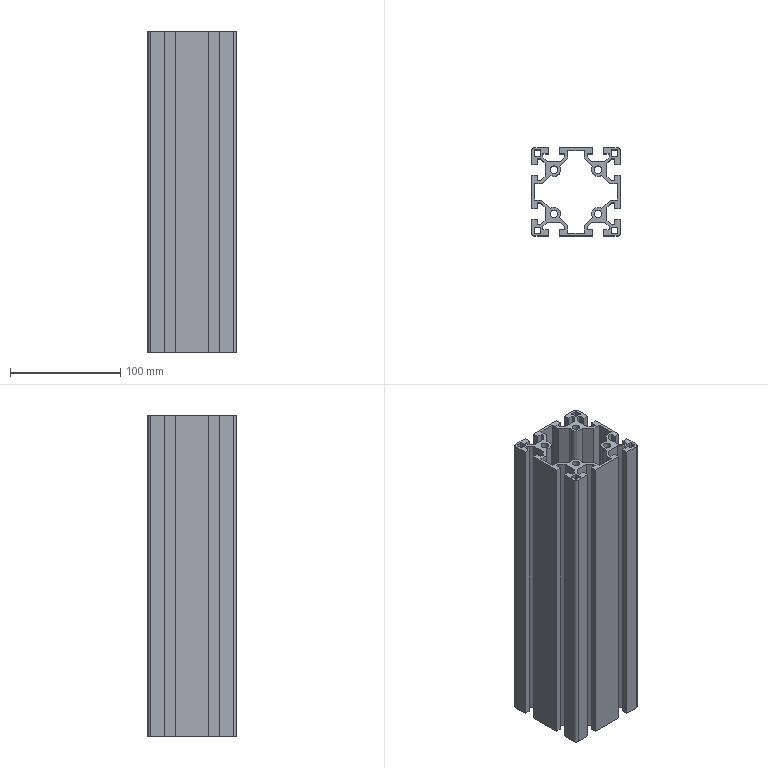Part | NX | 1 solid | 156 faces | box 80 x 80 x 290 mm | volume 508081 mm3 | plane 122 | cylinder 34 | commonest cylinder face diameters 2 x16 6.8 x8 11.8 x6 5.64 x4